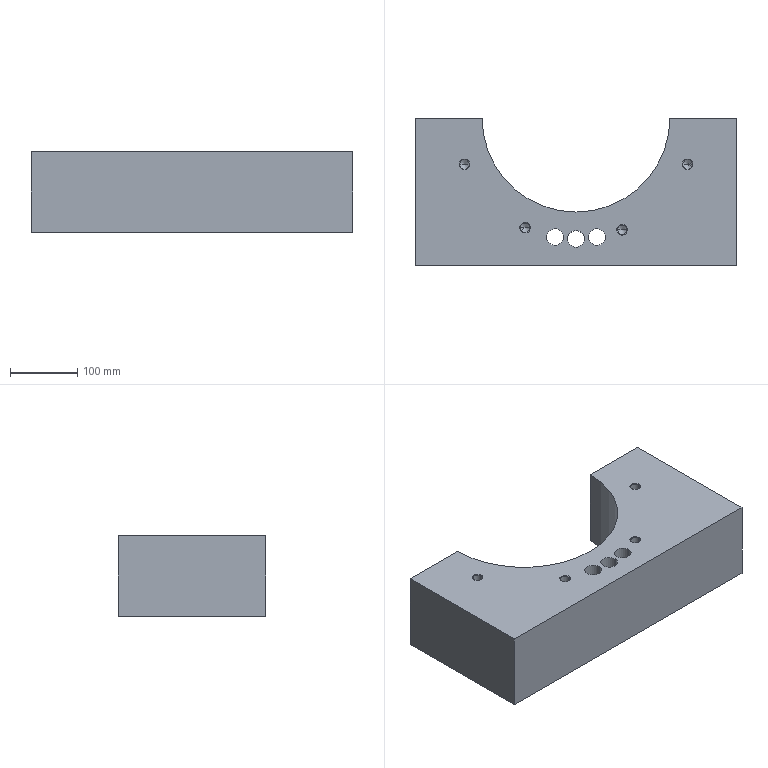Part | SolidWorks | features ICE 2, Extrusion 1, HoleWzd 1, RefAxis 1 | 1 solid | 38 faces | box 480 x 220 x 120 mm | volume 8780124 mm3 | cone 16 | cylinder 15 | plane 7 | commonest cylinder face diameters 14 x8 25 x6 280 x1
STEP:
#1=CARTESIAN_POINT('',(-173.298,41.117,119.14));
#2=VERTEX_POINT('',#1);
#3=CARTESIAN_POINT('',(-159.298,41.117,119.14));
#4=VERTEX_POINT('',#3);
#5=CARTESIAN_POINT('',(-166.298,41.117,119.14));
#6=DIRECTION('',(0.,0.,1.));
#7=DIRECTION('',(1.,0.,0.));
#8=AXIS2_PLACEMENT_3D('',#5,#6,#7);
#9=CIRCLE('',#8,7.);
#10=EDGE_CURVE('',#2,#4,#9,.T.);
#11=ORIENTED_EDGE('',*,*,#10,.F.);
#12=CARTESIAN_POINT('',(-174.323,41.117,120.));
#13=VERTEX_POINT('',#12);
#14=CARTESIAN_POINT('',(-174.323,41.117,120.));
#15=DIRECTION('',(-0.766,0.,0.6428));
#16=VECTOR('',#15,1000.);
#17=LINE('',#14,#16);
#18=EDGE_CURVE('',#2,#13,#17,.T.);
#19=ORIENTED_EDGE('',*,*,#18,.T.);
#20=CARTESIAN_POINT('',(-158.273,41.117,120.));
#21=VERTEX_POINT('',#20);
#22=CARTESIAN_POINT('',(-166.298,41.117,120.));
#23=DIRECTION('',(0.,0.,1.));
#24=DIRECTION('',(1.,0.,0.));
#25=AXIS2_PLACEMENT_3D('',#22,#23,#24);
#26=CIRCLE('',#25,8.025);
#27=EDGE_CURVE('',#13,#21,#26,.T.);
#28=ORIENTED_EDGE('',*,*,#27,.T.);
#29=CARTESIAN_POINT('',(-158.273,41.117,120.));
#30=DIRECTION('',(0.766,0.,0.6428));
#31=VECTOR('',#30,1000.);
#32=LINE('',#29,#31);
#33=EDGE_CURVE('',#4,#21,#32,.T.);
#34=ORIENTED_EDGE('',*,*,#33,.F.);
#35=EDGE_LOOP('',(#11,#19,#28,#34));
#36=FACE_OUTER_BOUND('',#35,.T.);
#37=CARTESIAN_POINT('',(-166.298,41.117,120.));
#38=DIRECTION('',(0.,0.,1.));
#39=DIRECTION('',(1.,0.,0.));
#40=AXIS2_PLACEMENT_3D('',#37,#38,#39);
#41=CONICAL_SURFACE('',#40,8.025,0.8727);
#42=ADVANCED_FACE('',(#36),#41,.F.);
#43=CARTESIAN_POINT('',(-173.298,41.117,88.));
#44=VERTEX_POINT('',#43);
#45=CARTESIAN_POINT('',(-159.298,41.117,88.));
#46=VERTEX_POINT('',#45);
#47=CARTESIAN_POINT('',(-166.298,41.117,88.));
#48=DIRECTION('',(0.,0.,1.));
#49=DIRECTION('',(1.,0.,0.));
#50=AXIS2_PLACEMENT_3D('',#47,#48,#49);
#51=CIRCLE('',#50,7.);
#52=EDGE_CURVE('',#44,#46,#51,.T.);
#53=ORIENTED_EDGE('',*,*,#52,.F.);
#54=CARTESIAN_POINT('',(-173.298,41.117,120.));
#55=DIRECTION('',(0.,0.,1.));
#56=VECTOR('',#55,1000.);
#57=LINE('',#54,#56);
#58=EDGE_CURVE('',#44,#2,#57,.T.);
#59=ORIENTED_EDGE('',*,*,#58,.T.);
#60=ORIENTED_EDGE('',*,*,#10,.T.);
#61=CARTESIAN_POINT('',(-159.298,41.117,120.));
#62=DIRECTION('',(0.,0.,1.));
#63=VECTOR('',#62,1000.);
#64=LINE('',#61,#63);
#65=EDGE_CURVE('',#46,#4,#64,.T.);
#66=ORIENTED_EDGE('',*,*,#65,.F.);
#67=EDGE_LOOP('',(#53,#59,#60,#66));
#68=FACE_OUTER_BOUND('',#67,.T.);
#69=CARTESIAN_POINT('',(-166.298,41.117,120.));
#70=DIRECTION('',(0.,0.,1.));
#71=DIRECTION('',(1.,0.,0.));
#72=AXIS2_PLACEMENT_3D('',#69,#70,#71);
#73=CYLINDRICAL_SURFACE('',#72,7.);
#74=ADVANCED_FACE('',(#68),#73,.F.);
#75=CARTESIAN_POINT('',(-166.298,41.117,83.794));
#76=VERTEX_POINT('',#75);
#77=CARTESIAN_POINT('',(-159.298,41.117,88.));
#78=DIRECTION('',(0.8572,0.,0.515));
#79=VECTOR('',#78,1000.);
#80=LINE('',#77,#79);
#81=EDGE_CURVE('',#76,#46,#80,.T.);
#82=ORIENTED_EDGE('',*,*,#81,.F.);
#83=CARTESIAN_POINT('',(-173.298,41.117,88.));
#84=DIRECTION('',(-0.8572,0.,0.515));
#85=VECTOR('',#84,1000.);
#86=LINE('',#83,#85);
#87=EDGE_CURVE('',#76,#44,#86,.T.);
#88=ORIENTED_EDGE('',*,*,#87,.T.);
#89=ORIENTED_EDGE('',*,*,#52,.T.);
#90=EDGE_LOOP('',(#82,#88,#89));
#91=FACE_OUTER_BOUND('',#90,.T.);
#92=CARTESIAN_POINT('',(-166.298,41.117,88.));
#93=DIRECTION('',(0.,0.,1.));
#94=DIRECTION('',(1.,0.,0.));
#95=AXIS2_PLACEMENT_3D('',#92,#93,#94);
#96=CONICAL_SURFACE('',#95,7.,1.03);
#97=ADVANCED_FACE('',(#91),#96,.F.);
#98=CARTESIAN_POINT('',(159.298,41.117,119.14));
#99=VERTEX_POINT('',#98);
#100=CARTESIAN_POINT('',(173.298,41.117,119.14));
#101=VERTEX_POINT('',#100);
#102=CARTESIAN_POINT('',(166.298,41.117,119.14));
#103=DIRECTION('',(0.,0.,1.));
#104=DIRECTION('',(1.,0.,0.));
#105=AXIS2_PLACEMENT_3D('',#102,#103,#104);
#106=CIRCLE('',#105,7.);
#107=EDGE_CURVE('',#99,#101,#106,.T.);
#108=ORIENTED_EDGE('',*,*,#107,.F.);
#109=CARTESIAN_POINT('',(158.273,41.117,120.));
#110=VERTEX_POINT('',#109);
#111=CARTESIAN_POINT('',(158.273,41.117,120.));
#112=DIRECTION('',(-0.766,0.,0.6428));
#113=VECTOR('',#112,1000.);
#114=LINE('',#111,#113);
#115=EDGE_CURVE('',#99,#110,#114,.T.);
#116=ORIENTED_EDGE('',*,*,#115,.T.);
#117=CARTESIAN_POINT('',(174.323,41.117,120.));
#118=VERTEX_POINT('',#117);
#119=CARTESIAN_POINT('',(166.298,41.117,120.));
#120=DIRECTION('',(0.,0.,1.));
#121=DIRECTION('',(1.,0.,0.));
#122=AXIS2_PLACEMENT_3D('',#119,#120,#121);
#123=CIRCLE('',#122,8.025);
#124=EDGE_CURVE('',#110,#118,#123,.T.);
#125=ORIENTED_EDGE('',*,*,#124,.T.);
#126=CARTESIAN_POINT('',(174.323,41.117,120.));
#127=DIRECTION('',(0.766,0.,0.6428));
#128=VECTOR('',#127,1000.);
#129=LINE('',#126,#128);
#130=EDGE_CURVE('',#101,#118,#129,.T.);
#131=ORIENTED_EDGE('',*,*,#130,.F.);
#132=EDGE_LOOP('',(#108,#116,#125,#131));
#133=FACE_OUTER_BOUND('',#132,.T.);
#134=CARTESIAN_POINT('',(166.298,41.117,120.));
#135=DIRECTION('',(0.,0.,1.));
#136=DIRECTION('',(1.,0.,0.));
#137=AXIS2_PLACEMENT_3D('',#134,#135,#136);
#138=CONICAL_SURFACE('',#137,8.025,0.8727);
#139=ADVANCED_FACE('',(#133),#138,.F.);
#140=CARTESIAN_POINT('',(159.298,41.117,88.));
#141=VERTEX_POINT('',#140);
#142=CARTESIAN_POINT('',(173.298,41.117,88.));
#143=VERTEX_POINT('',#142);
#144=CARTESIAN_POINT('',(166.298,41.117,88.));
#145=DIRECTION('',(0.,0.,1.));
#146=DIRECTION('',(1.,0.,0.));
#147=AXIS2_PLACEMENT_3D('',#144,#145,#146);
#148=CIRCLE('',#147,7.);
#149=EDGE_CURVE('',#141,#143,#148,.T.);
#150=ORIENTED_EDGE('',*,*,#149,.F.);
#151=CARTESIAN_POINT('',(159.298,41.117,120.));
#152=DIRECTION('',(0.,0.,1.));
#153=VECTOR('',#152,1000.);
#154=LINE('',#151,#153);
#155=EDGE_CURVE('',#141,#99,#154,.T.);
#156=ORIENTED_EDGE('',*,*,#155,.T.);
#157=ORIENTED_EDGE('',*,*,#107,.T.);
#158=CARTESIAN_POINT('',(173.298,41.117,120.));
#159=DIRECTION('',(0.,0.,1.));
#160=VECTOR('',#159,1000.);
#161=LINE('',#158,#160);
#162=EDGE_CURVE('',#143,#101,#161,.T.);
#163=ORIENTED_EDGE('',*,*,#162,.F.);
#164=EDGE_LOOP('',(#150,#156,#157,#163));
#165=FACE_OUTER_BOUND('',#164,.T.);
#166=CARTESIAN_POINT('',(166.298,41.117,120.));
#167=DIRECTION('',(0.,0.,1.));
#168=DIRECTION('',(1.,0.,0.));
#169=AXIS2_PLACEMENT_3D('',#166,#167,#168);
#170=CYLINDRICAL_SURFACE('',#169,7.);
#171=ADVANCED_FACE('',(#165),#170,.F.);
#172=CARTESIAN_POINT('',(166.298,41.117,83.794));
#173=VERTEX_POINT('',#172);
#174=CARTESIAN_POINT('',(173.298,41.117,88.));
#175=DIRECTION('',(0.8572,0.,0.515));
#176=VECTOR('',#175,1000.);
#177=LINE('',#174,#176);
#178=EDGE_CURVE('',#173,#143,#177,.T.);
#179=ORIENTED_EDGE('',*,*,#178,.F.);
#180=CARTESIAN_POINT('',(159.298,41.117,88.));
#181=DIRECTION('',(-0.8572,0.,0.515));
#182=VECTOR('',#181,1000.);
#183=LINE('',#180,#182);
#184=EDGE_CURVE('',#173,#141,#183,.T.);
#185=ORIENTED_EDGE('',*,*,#184,.T.);
#186=ORIENTED_EDGE('',*,*,#149,.T.);
#187=EDGE_LOOP('',(#179,#185,#186));
#188=FACE_OUTER_BOUND('',#187,.T.);
#189=CARTESIAN_POINT('',(166.298,41.117,88.));
#190=DIRECTION('',(0.,0.,1.));
#191=DIRECTION('',(1.,0.,0.));
#192=AXIS2_PLACEMENT_3D('',#189,#190,#191);
#193=CONICAL_SURFACE('',#192,7.,1.03);
#194=ADVANCED_FACE('',(#188),#193,.F.);
#195=CARTESIAN_POINT('',(61.883,-56.298,119.14));
#196=VERTEX_POINT('',#195);
#197=CARTESIAN_POINT('',(75.883,-56.298,119.14));
#198=VERTEX_POINT('',#197);
#199=CARTESIAN_POINT('',(68.883,-56.298,119.14));
#200=DIRECTION('',(0.,0.,1.));
#201=DIRECTION('',(1.,0.,0.));
#202=AXIS2_PLACEMENT_3D('',#199,#200,#201);
#203=CIRCLE('',#202,7.);
#204=EDGE_CURVE('',#196,#198,#203,.T.);
#205=ORIENTED_EDGE('',*,*,#204,.F.);
#206=CARTESIAN_POINT('',(60.858,-56.298,120.));
#207=VERTEX_POINT('',#206);
#208=CARTESIAN_POINT('',(60.858,-56.298,120.));
#209=DIRECTION('',(-0.766,0.,0.6428));
#210=VECTOR('',#209,1000.);
#211=LINE('',#208,#210);
#212=EDGE_CURVE('',#196,#207,#211,.T.);
#213=ORIENTED_EDGE('',*,*,#212,.T.);
#214=CARTESIAN_POINT('',(76.908,-56.298,120.));
#215=VERTEX_POINT('',#214);
#216=CARTESIAN_POINT('',(68.883,-56.298,120.));
#217=DIRECTION('',(0.,0.,1.));
#218=DIRECTION('',(1.,0.,0.));
#219=AXIS2_PLACEMENT_3D('',#216,#217,#218);
#220=CIRCLE('',#219,8.025);
#221=EDGE_CURVE('',#207,#215,#220,.T.);
#222=ORIENTED_EDGE('',*,*,#221,.T.);
#223=CARTESIAN_POINT('',(76.908,-56.298,120.));
#224=DIRECTION('',(0.766,0.,0.6428));
#225=VECTOR('',#224,1000.);
#226=LINE('',#223,#225);
#227=EDGE_CURVE('',#198,#215,#226,.T.);
#228=ORIENTED_EDGE('',*,*,#227,.F.);
#229=EDGE_LOOP('',(#205,#213,#222,#228));
#230=FACE_OUTER_BOUND('',#229,.T.);
#231=CARTESIAN_POINT('',(68.883,-56.298,120.));
#232=DIRECTION('',(0.,0.,1.));
#233=DIRECTION('',(1.,0.,0.));
#234=AXIS2_PLACEMENT_3D('',#231,#232,#233);
#235=CONICAL_SURFACE('',#234,8.025,0.8727);
#236=ADVANCED_FACE('',(#230),#235,.F.);
#237=CARTESIAN_POINT('',(61.883,-56.298,88.));
#238=VERTEX_POINT('',#237);
#239=CARTESIAN_POINT('',(75.883,-56.298,88.));
#240=VERTEX_POINT('',#239);
#241=CARTESIAN_POINT('',(68.883,-56.298,88.));
#242=DIRECTION('',(0.,0.,1.));
#243=DIRECTION('',(1.,0.,0.));
#244=AXIS2_PLACEMENT_3D('',#241,#242,#243);
#245=CIRCLE('',#244,7.);
#246=EDGE_CURVE('',#238,#240,#245,.T.);
#247=ORIENTED_EDGE('',*,*,#246,.F.);
#248=CARTESIAN_POINT('',(61.883,-56.298,120.));
#249=DIRECTION('',(0.,0.,1.));
#250=VECTOR('',#249,1000.);
#251=LINE('',#248,#250);
#252=EDGE_CURVE('',#238,#196,#251,.T.);
#253=ORIENTED_EDGE('',*,*,#252,.T.);
#254=ORIENTED_EDGE('',*,*,#204,.T.);
#255=CARTESIAN_POINT('',(75.883,-56.298,120.));
#256=DIRECTION('',(0.,0.,1.));
#257=VECTOR('',#256,1000.);
#258=LINE('',#255,#257);
#259=EDGE_CURVE('',#240,#198,#258,.T.);
#260=ORIENTED_EDGE('',*,*,#259,.F.);
#261=EDGE_LOOP('',(#247,#253,#254,#260));
#262=FACE_OUTER_BOUND('',#261,.T.);
#263=CARTESIAN_POINT('',(68.883,-56.298,120.));
#264=DIRECTION('',(0.,0.,1.));
#265=DIRECTION('',(1.,0.,0.));
#266=AXIS2_PLACEMENT_3D('',#263,#264,#265);
#267=CYLINDRICAL_SURFACE('',#266,7.);
#268=ADVANCED_FACE('',(#262),#267,.F.);
#269=CARTESIAN_POINT('',(68.883,-56.298,83.794));
#270=VERTEX_POINT('',#269);
#271=CARTESIAN_POINT('',(75.883,-56.298,88.));
#272=DIRECTION('',(0.8572,0.,0.515));
#273=VECTOR('',#272,1000.);
#274=LINE('',#271,#273);
#275=EDGE_CURVE('',#270,#240,#274,.T.);
#276=ORIENTED_EDGE('',*,*,#275,.F.);
#277=CARTESIAN_POINT('',(61.883,-56.298,88.));
#278=DIRECTION('',(-0.8572,0.,0.515));
#279=VECTOR('',#278,1000.);
#280=LINE('',#277,#279);
#281=EDGE_CURVE('',#270,#238,#280,.T.);
#282=ORIENTED_EDGE('',*,*,#281,.T.);
#283=ORIENTED_EDGE('',*,*,#246,.T.);
#284=EDGE_LOOP('',(#276,#282,#283));
#285=FACE_OUTER_BOUND('',#284,.T.);
#286=CARTESIAN_POINT('',(68.883,-56.298,88.));
#287=DIRECTION('',(0.,0.,1.));
#288=DIRECTION('',(1.,0.,0.));
#289=AXIS2_PLACEMENT_3D('',#286,#287,#288);
#290=CONICAL_SURFACE('',#289,7.,1.03);
#291=ADVANCED_FACE('',(#285),#290,.F.);
#292=CARTESIAN_POINT('',(-82.868,-53.23,119.14));
#293=VERTEX_POINT('',#292);
#294=CARTESIAN_POINT('',(-68.868,-53.23,119.14));
#295=VERTEX_POINT('',#294);
#296=CARTESIAN_POINT('',(-75.868,-53.23,119.14));
#297=DIRECTION('',(0.,0.,1.));
#298=DIRECTION('',(1.,0.,0.));
#299=AXIS2_PLACEMENT_3D('',#296,#297,#298);
#300=CIRCLE('',#299,7.);
#301=EDGE_CURVE('',#293,#295,#300,.T.);
#302=ORIENTED_EDGE('',*,*,#301,.F.);
#303=CARTESIAN_POINT('',(-83.893,-53.23,120.));
#304=VERTEX_POINT('',#303);
#305=CARTESIAN_POINT('',(-83.893,-53.23,120.));
#306=DIRECTION('',(-0.766,0.,0.6428));
#307=VECTOR('',#306,1000.);
#308=LINE('',#305,#307);
#309=EDGE_CURVE('',#293,#304,#308,.T.);
#310=ORIENTED_EDGE('',*,*,#309,.T.);
#311=CARTESIAN_POINT('',(-67.843,-53.23,120.));
#312=VERTEX_POINT('',#311);
#313=CARTESIAN_POINT('',(-75.868,-53.23,120.));
#314=DIRECTION('',(0.,0.,1.));
#315=DIRECTION('',(1.,0.,0.));
#316=AXIS2_PLACEMENT_3D('',#313,#314,#315);
#317=CIRCLE('',#316,8.025);
#318=EDGE_CURVE('',#304,#312,#317,.T.);
#319=ORIENTED_EDGE('',*,*,#318,.T.);
#320=CARTESIAN_POINT('',(-67.843,-53.23,120.));
#321=DIRECTION('',(0.766,0.,0.6428));
#322=VECTOR('',#321,1000.);
#323=LINE('',#320,#322);
#324=EDGE_CURVE('',#295,#312,#323,.T.);
#325=ORIENTED_EDGE('',*,*,#324,.F.);
#326=EDGE_LOOP('',(#302,#310,#319,#325));
#327=FACE_OUTER_BOUND('',#326,.T.);
#328=CARTESIAN_POINT('',(-75.868,-53.23,120.));
#329=DIRECTION('',(0.,0.,1.));
#330=DIRECTION('',(1.,0.,0.));
#331=AXIS2_PLACEMENT_3D('',#328,#329,#330);
#332=CONICAL_SURFACE('',#331,8.025,0.8727);
#333=ADVANCED_FACE('',(#327),#332,.F.);
#334=CARTESIAN_POINT('',(-82.868,-53.23,88.));
#335=VERTEX_POINT('',#334);
#336=CARTESIAN_POINT('',(-68.868,-53.23,88.));
#337=VERTEX_POINT('',#336);
#338=CARTESIAN_POINT('',(-75.868,-53.23,88.));
#339=DIRECTION('',(0.,0.,1.));
#340=DIRECTION('',(1.,0.,0.));
#341=AXIS2_PLACEMENT_3D('',#338,#339,#340);
#342=CIRCLE('',#341,7.);
#343=EDGE_CURVE('',#335,#337,#342,.T.);
#344=ORIENTED_EDGE('',*,*,#343,.F.);
#345=CARTESIAN_POINT('',(-82.868,-53.23,120.));
#346=DIRECTION('',(0.,0.,1.));
#347=VECTOR('',#346,1000.);
#348=LINE('',#345,#347);
#349=EDGE_CURVE('',#335,#293,#348,.T.);
#350=ORIENTED_EDGE('',*,*,#349,.T.);
#351=ORIENTED_EDGE('',*,*,#301,.T.);
#352=CARTESIAN_POINT('',(-68.868,-53.23,120.));
#353=DIRECTION('',(0.,0.,1.));
#354=VECTOR('',#353,1000.);
#355=LINE('',#352,#354);
#356=EDGE_CURVE('',#337,#295,#355,.T.);
#357=ORIENTED_EDGE('',*,*,#356,.F.);
#358=EDGE_LOOP('',(#344,#350,#351,#357));
#359=FACE_OUTER_BOUND('',#358,.T.);
#360=CARTESIAN_POINT('',(-75.868,-53.23,120.));
#361=DIRECTION('',(0.,0.,1.));
#362=DIRECTION('',(1.,0.,0.));
#363=AXIS2_PLACEMENT_3D('',#360,#361,#362);
#364=CYLINDRICAL_SURFACE('',#363,7.);
#365=ADVANCED_FACE('',(#359),#364,.F.);
#366=CARTESIAN_POINT('',(-75.868,-53.23,83.794));
#367=VERTEX_POINT('',#366);
#368=CARTESIAN_POINT('',(-68.868,-53.23,88.));
#369=DIRECTION('',(0.8572,0.,0.515));
#370=VECTOR('',#369,1000.);
#371=LINE('',#368,#370);
#372=EDGE_CURVE('',#367,#337,#371,.T.);
#373=ORIENTED_EDGE('',*,*,#372,.F.);
#374=CARTESIAN_POINT('',(-82.868,-53.23,88.));
#375=DIRECTION('',(-0.8572,0.,0.515));
#376=VECTOR('',#375,1000.);
#377=LINE('',#374,#376);
#378=EDGE_CURVE('',#367,#335,#377,.T.);
#379=ORIENTED_EDGE('',*,*,#378,.T.);
#380=ORIENTED_EDGE('',*,*,#343,.T.);
#381=EDGE_LOOP('',(#373,#379,#380));
#382=FACE_OUTER_BOUND('',#381,.T.);
#383=CARTESIAN_POINT('',(-75.868,-53.23,88.));
#384=DIRECTION('',(0.,0.,1.));
#385=DIRECTION('',(1.,0.,0.));
#386=AXIS2_PLACEMENT_3D('',#383,#384,#385);
#387=CONICAL_SURFACE('',#386,7.,1.03);
#388=ADVANCED_FACE('',(#382),#387,.F.);
#389=CARTESIAN_POINT('',(18.757,-67.265,0.));
#390=VERTEX_POINT('',#389);
#391=CARTESIAN_POINT('',(43.757,-67.265,0.));
#392=VERTEX_POINT('',#391);
#393=CARTESIAN_POINT('',(31.257,-67.265,0.));
#394=DIRECTION('',(0.,0.,1.));
#395=DIRECTION('',(-1.,0.,0.));
#396=AXIS2_PLACEMENT_3D('',#393,#394,#395);
#397=CIRCLE('',#396,12.5);
#398=EDGE_CURVE('',#390,#392,#397,.T.);
#399=ORIENTED_EDGE('',*,*,#398,.F.);
#400=CARTESIAN_POINT('',(18.757,-67.265,120.));
#401=VERTEX_POINT('',#400);
#402=CARTESIAN_POINT('',(18.757,-67.265,0.));
#403=DIRECTION('',(0.,0.,1.));
#404=VECTOR('',#403,1000.);
#405=LINE('',#402,#404);
#406=EDGE_CURVE('',#390,#401,#405,.T.);
#407=ORIENTED_EDGE('',*,*,#406,.T.);
#408=CARTESIAN_POINT('',(43.757,-67.265,120.));
#409=VERTEX_POINT('',#408);
#410=CARTESIAN_POINT('',(31.257,-67.265,120.));
#411=DIRECTION('',(0.,0.,1.));
#412=DIRECTION('',(1.,0.,0.));
#413=AXIS2_PLACEMENT_3D('',#410,#411,#412);
#414=CIRCLE('',#413,12.5);
#415=EDGE_CURVE('',#401,#409,#414,.T.);
#416=ORIENTED_EDGE('',*,*,#415,.T.);
#417=CARTESIAN_POINT('',(43.757,-67.265,0.));
#418=DIRECTION('',(0.,0.,1.));
#419=VECTOR('',#418,1000.);
#420=LINE('',#417,#419);
#421=EDGE_CURVE('',#392,#409,#420,.T.);
#422=ORIENTED_EDGE('',*,*,#421,.F.);
#423=EDGE_LOOP('',(#399,#407,#416,#422));
#424=FACE_OUTER_BOUND('',#423,.T.);
#425=CARTESIAN_POINT('',(31.257,-67.265,0.));
#426=DIRECTION('',(0.,0.,1.));
#427=DIRECTION('',(1.,0.,0.));
#428=AXIS2_PLACEMENT_3D('',#425,#426,#427);
#429=CYLINDRICAL_SURFACE('',#428,12.5);
#430=ADVANCED_FACE('',(#424),#429,.F.);
#431=CARTESIAN_POINT('',(-43.757,-67.265,0.));
#432=VERTEX_POINT('',#431);
#433=CARTESIAN_POINT('',(-18.757,-67.265,0.));
#434=VERTEX_POINT('',#433);
#435=CARTESIAN_POINT('',(-31.257,-67.265,0.));
#436=DIRECTION('',(0.,0.,1.));
#437=DIRECTION('',(1.,0.,0.));
#438=AXIS2_PLACEMENT_3D('',#435,#436,#437);
#439=CIRCLE('',#438,12.5);
#440=EDGE_CURVE('',#432,#434,#439,.T.);
#441=ORIENTED_EDGE('',*,*,#440,.F.);
#442=CARTESIAN_POINT('',(-43.757,-67.265,120.));
#443=VERTEX_POINT('',#442);
#444=CARTESIAN_POINT('',(-43.757,-67.265,0.));
#445=DIRECTION('',(0.,0.,1.));
#446=VECTOR('',#445,1000.);
#447=LINE('',#444,#446);
#448=EDGE_CURVE('',#432,#443,#447,.T.);
#449=ORIENTED_EDGE('',*,*,#448,.T.);
#450=CARTESIAN_POINT('',(-18.757,-67.265,120.));
#451=VERTEX_POINT('',#450);
#452=CARTESIAN_POINT('',(-31.257,-67.265,120.));
#453=DIRECTION('',(0.,0.,1.));
#454=DIRECTION('',(1.,0.,0.));
#455=AXIS2_PLACEMENT_3D('',#452,#453,#454);
#456=CIRCLE('',#455,12.5);
#457=EDGE_CURVE('',#443,#451,#456,.T.);
#458=ORIENTED_EDGE('',*,*,#457,.T.);
#459=CARTESIAN_POINT('',(-18.757,-67.265,0.));
#460=DIRECTION('',(0.,0.,1.));
#461=VECTOR('',#460,1000.);
#462=LINE('',#459,#461);
#463=EDGE_CURVE('',#434,#451,#462,.T.);
#464=ORIENTED_EDGE('',*,*,#463,.F.);
#465=EDGE_LOOP('',(#441,#449,#458,#464));
#466=FACE_OUTER_BOUND('',#465,.T.);
#467=CARTESIAN_POINT('',(-31.257,-67.265,0.));
#468=DIRECTION('',(0.,0.,1.));
#469=DIRECTION('',(1.,0.,0.));
#470=AXIS2_PLACEMENT_3D('',#467,#468,#469);
#471=CYLINDRICAL_SURFACE('',#470,12.5);
#472=ADVANCED_FACE('',(#466),#471,.F.);
#473=CARTESIAN_POINT('',(-12.5,-70.,0.));
#474=VERTEX_POINT('',#473);
#475=CARTESIAN_POINT('',(12.5,-70.,0.));
#476=VERTEX_POINT('',#475);
#477=CARTESIAN_POINT('',(0.,-70.,0.));
#478=DIRECTION('',(0.,0.,1.));
#479=DIRECTION('',(1.,0.,0.));
#480=AXIS2_PLACEMENT_3D('',#477,#478,#479);
#481=CIRCLE('',#480,12.5);
#482=EDGE_CURVE('',#474,#476,#481,.T.);
#483=ORIENTED_EDGE('',*,*,#482,.F.);
#484=CARTESIAN_POINT('',(-12.5,-70.,120.));
#485=VERTEX_POINT('',#484);
#486=CARTESIAN_POINT('',(-12.5,-70.,0.));
#487=DIRECTION('',(0.,0.,1.));
#488=VECTOR('',#487,1000.);
#489=LINE('',#486,#488);
#490=EDGE_CURVE('',#474,#485,#489,.T.);
#491=ORIENTED_EDGE('',*,*,#490,.T.);
#492=CARTESIAN_POINT('',(12.5,-70.,120.));
#493=VERTEX_POINT('',#492);
#494=CARTESIAN_POINT('',(0.,-70.,120.));
#495=DIRECTION('',(0.,0.,1.));
#496=DIRECTION('',(1.,0.,0.));
#497=AXIS2_PLACEMENT_3D('',#494,#495,#496);
#498=CIRCLE('',#497,12.5);
#499=EDGE_CURVE('',#485,#493,#498,.T.);
#500=ORIENTED_EDGE('',*,*,#499,.T.);
#501=CARTESIAN_POINT('',(12.5,-70.,0.));
#502=DIRECTION('',(0.,0.,1.));
#503=VECTOR('',#502,1000.);
#504=LINE('',#501,#503);
#505=EDGE_CURVE('',#476,#493,#504,.T.);
#506=ORIENTED_EDGE('',*,*,#505,.F.);
#507=EDGE_LOOP('',(#483,#491,#500,#506));
#508=FACE_OUTER_BOUND('',#507,.T.);
#509=CARTESIAN_POINT('',(0.,-70.,0.));
#510=DIRECTION('',(0.,0.,1.));
#511=DIRECTION('',(1.,0.,0.));
#512=AXIS2_PLACEMENT_3D('',#509,#510,#511);
#513=CYLINDRICAL_SURFACE('',#512,12.5);
#514=ADVANCED_FACE('',(#508),#513,.F.);
#515=CARTESIAN_POINT('',(240.,110.,0.));
#516=VERTEX_POINT('',#515);
#517=CARTESIAN_POINT('',(140.,110.,0.));
#518=VERTEX_POINT('',#517);
#519=CARTESIAN_POINT('',(-240.,110.,0.));
#520=DIRECTION('',(-1.,0.,0.));
#521=VECTOR('',#520,1000.);
#522=LINE('',#519,#521);
#523=EDGE_CURVE('',#516,#518,#522,.T.);
#524=ORIENTED_EDGE('',*,*,#523,.T.);
#525=CARTESIAN_POINT('',(140.,110.,120.));
#526=VERTEX_POINT('',#525);
#527=CARTESIAN_POINT('',(140.,110.,0.));
#528=DIRECTION('',(0.,0.,1.));
#529=VECTOR('',#528,1000.);
#530=LINE('',#527,#529);
#531=EDGE_CURVE('',#518,#526,#530,.T.);
#532=ORIENTED_EDGE('',*,*,#531,.T.);
#533=CARTESIAN_POINT('',(240.,110.,120.));
#534=VERTEX_POINT('',#533);
#535=CARTESIAN_POINT('',(-240.,110.,120.));
#536=DIRECTION('',(-1.,0.,0.));
#537=VECTOR('',#536,1000.);
#538=LINE('',#535,#537);
#539=EDGE_CURVE('',#534,#526,#538,.T.);
#540=ORIENTED_EDGE('',*,*,#539,.F.);
#541=CARTESIAN_POINT('',(240.,110.,120.));
#542=DIRECTION('',(0.,0.,-1.));
#543=VECTOR('',#542,1000.);
#544=LINE('',#541,#543);
#545=EDGE_CURVE('',#534,#516,#544,.T.);
#546=ORIENTED_EDGE('',*,*,#545,.T.);
#547=EDGE_LOOP('',(#524,#532,#540,#546));
#548=FACE_OUTER_BOUND('',#547,.T.);
#549=CARTESIAN_POINT('',(-240.,110.,120.));
#550=DIRECTION('',(0.,-1.,0.));
#551=DIRECTION('',(0.,0.,-1.));
#552=AXIS2_PLACEMENT_3D('',#549,#550,#551);
#553=PLANE('',#552);
#554=ADVANCED_FACE('',(#548),#553,.F.);
#555=CARTESIAN_POINT('',(240.,-110.,0.));
#556=VERTEX_POINT('',#555);
#557=CARTESIAN_POINT('',(240.,110.,0.));
#558=DIRECTION('',(0.,1.,0.));
#559=VECTOR('',#558,1000.);
#560=LINE('',#557,#559);
#561=EDGE_CURVE('',#556,#516,#560,.T.);
#562=ORIENTED_EDGE('',*,*,#561,.T.);
#563=ORIENTED_EDGE('',*,*,#545,.F.);
#564=CARTESIAN_POINT('',(240.,-110.,120.));
#565=VERTEX_POINT('',#564);
#566=CARTESIAN_POINT('',(240.,110.,120.));
#567=DIRECTION('',(0.,1.,0.));
#568=VECTOR('',#567,1000.);
#569=LINE('',#566,#568);
#570=EDGE_CURVE('',#565,#534,#569,.T.);
#571=ORIENTED_EDGE('',*,*,#570,.F.);
#572=CARTESIAN_POINT('',(240.,-110.,120.));
#573=DIRECTION('',(0.,0.,-1.));
#574=VECTOR('',#573,1000.);
#575=LINE('',#572,#574);
#576=EDGE_CURVE('',#565,#556,#575,.T.);
#577=ORIENTED_EDGE('',*,*,#576,.T.);
#578=EDGE_LOOP('',(#562,#563,#571,#577));
#579=FACE_OUTER_BOUND('',#578,.T.);
#580=CARTESIAN_POINT('',(240.,110.,120.));
#581=DIRECTION('',(-1.,0.,0.));
#582=DIRECTION('',(0.,0.,1.));
#583=AXIS2_PLACEMENT_3D('',#580,#581,#582);
#584=PLANE('',#583);
#585=ADVANCED_FACE('',(#579),#584,.F.);
#586=CARTESIAN_POINT('',(-140.,110.,120.));
#587=VERTEX_POINT('',#586);
#588=CARTESIAN_POINT('',(-240.,110.,120.));
#589=VERTEX_POINT('',#588);
#590=CARTESIAN_POINT('',(-240.,110.,120.));
#591=DIRECTION('',(-1.,0.,0.));
#592=VECTOR('',#591,1000.);
#593=LINE('',#590,#592);
#594=EDGE_CURVE('',#587,#589,#593,.T.);
#595=ORIENTED_EDGE('',*,*,#594,.F.);
#596=CARTESIAN_POINT('',(-140.,110.,0.));
#597=VERTEX_POINT('',#596);
#598=CARTESIAN_POINT('',(-140.,110.,0.));
#599=DIRECTION('',(0.,0.,-1.));
#600=VECTOR('',#599,1000.);
#601=LINE('',#598,#600);
#602=EDGE_CURVE('',#587,#597,#601,.T.);
#603=ORIENTED_EDGE('',*,*,#602,.T.);
#604=CARTESIAN_POINT('',(-240.,110.,0.));
#605=VERTEX_POINT('',#604);
#606=CARTESIAN_POINT('',(-240.,110.,0.));
#607=DIRECTION('',(-1.,0.,0.));
#608=VECTOR('',#607,1000.);
#609=LINE('',#606,#608);
#610=EDGE_CURVE('',#597,#605,#609,.T.);
#611=ORIENTED_EDGE('',*,*,#610,.T.);
#612=CARTESIAN_POINT('',(-240.,110.,120.));
#613=DIRECTION('',(0.,0.,-1.));
#614=VECTOR('',#613,1000.);
#615=LINE('',#612,#614);
#616=EDGE_CURVE('',#589,#605,#615,.T.);
#617=ORIENTED_EDGE('',*,*,#616,.F.);
#618=EDGE_LOOP('',(#595,#603,#611,#617));
#619=FACE_OUTER_BOUND('',#618,.T.);
#620=CARTESIAN_POINT('',(-240.,110.,120.));
#621=DIRECTION('',(0.,-1.,0.));
#622=DIRECTION('',(0.,0.,-1.));
#623=AXIS2_PLACEMENT_3D('',#620,#621,#622);
#624=PLANE('',#623);
#625=ADVANCED_FACE('',(#619),#624,.F.);
#626=CARTESIAN_POINT('',(-240.,-110.,0.));
#627=VERTEX_POINT('',#626);
#628=CARTESIAN_POINT('',(-240.,110.,0.));
#629=DIRECTION('',(0.,-1.,0.));
#630=VECTOR('',#629,1000.);
#631=LINE('',#628,#630);
#632=EDGE_CURVE('',#605,#627,#631,.T.);
#633=ORIENTED_EDGE('',*,*,#632,.T.);
#634=CARTESIAN_POINT('',(-240.,-110.,120.));
#635=VERTEX_POINT('',#634);
#636=CARTESIAN_POINT('',(-240.,-110.,120.));
#637=DIRECTION('',(0.,0.,-1.));
#638=VECTOR('',#637,1000.);
#639=LINE('',#636,#638);
#640=EDGE_CURVE('',#635,#627,#639,.T.);
#641=ORIENTED_EDGE('',*,*,#640,.F.);
#642=CARTESIAN_POINT('',(-240.,110.,120.));
#643=DIRECTION('',(0.,-1.,0.));
#644=VECTOR('',#643,1000.);
#645=LINE('',#642,#644);
#646=EDGE_CURVE('',#589,#635,#645,.T.);
#647=ORIENTED_EDGE('',*,*,#646,.F.);
#648=ORIENTED_EDGE('',*,*,#616,.T.);
#649=EDGE_LOOP('',(#633,#641,#647,#648));
#650=FACE_OUTER_BOUND('',#649,.T.);
#651=CARTESIAN_POINT('',(-240.,110.,120.));
#652=DIRECTION('',(1.,0.,0.));
#653=DIRECTION('',(0.,0.,-1.));
#654=AXIS2_PLACEMENT_3D('',#651,#652,#653);
#655=PLANE('',#654);
#656=ADVANCED_FACE('',(#650),#655,.F.);
#657=CARTESIAN_POINT('',(-240.,-110.,0.));
#658=DIRECTION('',(1.,0.,0.));
#659=VECTOR('',#658,1000.);
#660=LINE('',#657,#659);
#661=EDGE_CURVE('',#627,#556,#660,.T.);
#662=ORIENTED_EDGE('',*,*,#661,.T.);
#663=ORIENTED_EDGE('',*,*,#576,.F.);
#664=CARTESIAN_POINT('',(-240.,-110.,120.));
#665=DIRECTION('',(1.,0.,0.));
#666=VECTOR('',#665,1000.);
#667=LINE('',#664,#666);
#668=EDGE_CURVE('',#635,#565,#667,.T.);
#669=ORIENTED_EDGE('',*,*,#668,.F.);
#670=ORIENTED_EDGE('',*,*,#640,.T.);
#671=EDGE_LOOP('',(#662,#663,#669,#670));
#672=FACE_OUTER_BOUND('',#671,.T.);
#673=CARTESIAN_POINT('',(-240.,-110.,120.));
#674=DIRECTION('',(0.,1.,0.));
#675=DIRECTION('',(0.,0.,1.));
#676=AXIS2_PLACEMENT_3D('',#673,#674,#675);
#677=PLANE('',#676);
#678=ADVANCED_FACE('',(#672),#677,.F.);
#679=CARTESIAN_POINT('',(-166.298,41.117,120.));
#680=DIRECTION('',(0.,0.,1.));
#681=DIRECTION('',(1.,0.,0.));
#682=AXIS2_PLACEMENT_3D('',#679,#680,#681);
#683=CIRCLE('',#682,8.025);
#684=EDGE_CURVE('',#21,#13,#683,.T.);
#685=ORIENTED_EDGE('',*,*,#684,.F.);
#686=ORIENTED_EDGE('',*,*,#27,.F.);
#687=EDGE_LOOP('',(#685,#686));
#688=FACE_BOUND('',#687,.T.);
#689=CARTESIAN_POINT('',(166.298,41.117,120.));
#690=DIRECTION('',(0.,0.,1.));
#691=DIRECTION('',(1.,0.,0.));
#692=AXIS2_PLACEMENT_3D('',#689,#690,#691);
#693=CIRCLE('',#692,8.025);
#694=EDGE_CURVE('',#118,#110,#693,.T.);
#695=ORIENTED_EDGE('',*,*,#694,.F.);
#696=ORIENTED_EDGE('',*,*,#124,.F.);
#697=EDGE_LOOP('',(#695,#696));
#698=FACE_BOUND('',#697,.T.);
#699=CARTESIAN_POINT('',(68.883,-56.298,120.));
#700=DIRECTION('',(0.,0.,1.));
#701=DIRECTION('',(1.,0.,0.));
#702=AXIS2_PLACEMENT_3D('',#699,#700,#701);
#703=CIRCLE('',#702,8.025);
#704=EDGE_CURVE('',#215,#207,#703,.T.);
#705=ORIENTED_EDGE('',*,*,#704,.F.);
#706=ORIENTED_EDGE('',*,*,#221,.F.);
#707=EDGE_LOOP('',(#705,#706));
#708=FACE_BOUND('',#707,.T.);
#709=CARTESIAN_POINT('',(-75.868,-53.23,120.));
#710=DIRECTION('',(0.,0.,1.));
#711=DIRECTION('',(1.,0.,0.));
#712=AXIS2_PLACEMENT_3D('',#709,#710,#711);
#713=CIRCLE('',#712,8.025);
#714=EDGE_CURVE('',#312,#304,#713,.T.);
#715=ORIENTED_EDGE('',*,*,#714,.F.);
#716=ORIENTED_EDGE('',*,*,#318,.F.);
#717=EDGE_LOOP('',(#715,#716));
#718=FACE_BOUND('',#717,.T.);
#719=CARTESIAN_POINT('',(31.257,-67.265,120.));
#720=DIRECTION('',(0.,0.,1.));
#721=DIRECTION('',(1.,0.,0.));
#722=AXIS2_PLACEMENT_3D('',#719,#720,#721);
#723=CIRCLE('',#722,12.5);
#724=EDGE_CURVE('',#409,#401,#723,.T.);
#725=ORIENTED_EDGE('',*,*,#724,.F.);
#726=ORIENTED_EDGE('',*,*,#415,.F.);
#727=EDGE_LOOP('',(#725,#726));
#728=FACE_BOUND('',#727,.T.);
#729=CARTESIAN_POINT('',(-31.257,-67.265,120.));
#730=DIRECTION('',(0.,0.,1.));
#731=DIRECTION('',(1.,0.,0.));
#732=AXIS2_PLACEMENT_3D('',#729,#730,#731);
#733=CIRCLE('',#732,12.5);
#734=EDGE_CURVE('',#451,#443,#733,.T.);
#735=ORIENTED_EDGE('',*,*,#734,.F.);
#736=ORIENTED_EDGE('',*,*,#457,.F.);
#737=EDGE_LOOP('',(#735,#736));
#738=FACE_BOUND('',#737,.T.);
#739=CARTESIAN_POINT('',(0.,-70.,120.));
#740=DIRECTION('',(0.,0.,1.));
#741=DIRECTION('',(1.,0.,0.));
#742=AXIS2_PLACEMENT_3D('',#739,#740,#741);
#743=CIRCLE('',#742,12.5);
#744=EDGE_CURVE('',#493,#485,#743,.T.);
#745=ORIENTED_EDGE('',*,*,#744,.F.);
#746=ORIENTED_EDGE('',*,*,#499,.F.);
#747=EDGE_LOOP('',(#745,#746));
#748=FACE_BOUND('',#747,.T.);
#749=CARTESIAN_POINT('',(0.,110.,120.));
#750=DIRECTION('',(0.,0.,1.));
#751=DIRECTION('',(1.,0.,0.));
#752=AXIS2_PLACEMENT_3D('',#749,#750,#751);
#753=CIRCLE('',#752,140.);
#754=EDGE_CURVE('',#587,#526,#753,.T.);
#755=ORIENTED_EDGE('',*,*,#754,.F.);
#756=ORIENTED_EDGE('',*,*,#594,.T.);
#757=ORIENTED_EDGE('',*,*,#646,.T.);
#758=ORIENTED_EDGE('',*,*,#668,.T.);
#759=ORIENTED_EDGE('',*,*,#570,.T.);
#760=ORIENTED_EDGE('',*,*,#539,.T.);
#761=EDGE_LOOP('',(#755,#756,#757,#758,#759,#760));
#762=FACE_OUTER_BOUND('',#761,.T.);
#763=CARTESIAN_POINT('',(0.,0.,120.));
#764=DIRECTION('',(0.,0.,1.));
#765=DIRECTION('',(1.,0.,0.));
#766=AXIS2_PLACEMENT_3D('',#763,#764,#765);
#767=PLANE('',#766);
#768=ADVANCED_FACE('',(#688,#698,#708,#718,#728,#738,#748,#762),#767,.T.);
#769=CARTESIAN_POINT('',(31.257,-67.265,0.));
#770=DIRECTION('',(0.,0.,1.));
#771=DIRECTION('',(-1.,0.,0.));
#772=AXIS2_PLACEMENT_3D('',#769,#770,#771);
#773=CIRCLE('',#772,12.5);
#774=EDGE_CURVE('',#392,#390,#773,.T.);
#775=ORIENTED_EDGE('',*,*,#774,.T.);
#776=ORIENTED_EDGE('',*,*,#398,.T.);
#777=EDGE_LOOP('',(#775,#776));
#778=FACE_BOUND('',#777,.T.);
#779=CARTESIAN_POINT('',(-31.257,-67.265,0.));
#780=DIRECTION('',(0.,0.,1.));
#781=DIRECTION('',(1.,0.,0.));
#782=AXIS2_PLACEMENT_3D('',#779,#780,#781);
#783=CIRCLE('',#782,12.5);
#784=EDGE_CURVE('',#434,#432,#783,.T.);
#785=ORIENTED_EDGE('',*,*,#784,.T.);
#786=ORIENTED_EDGE('',*,*,#440,.T.);
#787=EDGE_LOOP('',(#785,#786));
#788=FACE_BOUND('',#787,.T.);
#789=CARTESIAN_POINT('',(0.,-70.,0.));
#790=DIRECTION('',(0.,0.,1.));
#791=DIRECTION('',(1.,0.,0.));
#792=AXIS2_PLACEMENT_3D('',#789,#790,#791);
#793=CIRCLE('',#792,12.5);
#794=EDGE_CURVE('',#476,#474,#793,.T.);
#795=ORIENTED_EDGE('',*,*,#794,.T.);
#796=ORIENTED_EDGE('',*,*,#482,.T.);
#797=EDGE_LOOP('',(#795,#796));
#798=FACE_BOUND('',#797,.T.);
#799=ORIENTED_EDGE('',*,*,#610,.F.);
#800=CARTESIAN_POINT('',(0.,110.,0.));
#801=DIRECTION('',(0.,0.,1.));
#802=DIRECTION('',(1.,0.,0.));
#803=AXIS2_PLACEMENT_3D('',#800,#801,#802);
#804=CIRCLE('',#803,140.);
#805=EDGE_CURVE('',#597,#518,#804,.T.);
#806=ORIENTED_EDGE('',*,*,#805,.T.);
#807=ORIENTED_EDGE('',*,*,#523,.F.);
#808=ORIENTED_EDGE('',*,*,#561,.F.);
#809=ORIENTED_EDGE('',*,*,#661,.F.);
#810=ORIENTED_EDGE('',*,*,#632,.F.);
#811=EDGE_LOOP('',(#799,#806,#807,#808,#809,#810));
#812=FACE_OUTER_BOUND('',#811,.T.);
#813=CARTESIAN_POINT('',(0.,0.,0.));
#814=DIRECTION('',(0.,0.,1.));
#815=DIRECTION('',(1.,0.,0.));
#816=AXIS2_PLACEMENT_3D('',#813,#814,#815);
#817=PLANE('',#816);
#818=ADVANCED_FACE('',(#778,#788,#798,#812),#817,.F.);
#819=ORIENTED_EDGE('',*,*,#805,.F.);
#820=ORIENTED_EDGE('',*,*,#602,.F.);
#821=ORIENTED_EDGE('',*,*,#754,.T.);
#822=ORIENTED_EDGE('',*,*,#531,.F.);
#823=EDGE_LOOP('',(#819,#820,#821,#822));
#824=FACE_OUTER_BOUND('',#823,.T.);
#825=CARTESIAN_POINT('',(0.,110.,0.));
#826=DIRECTION('',(0.,0.,1.));
#827=DIRECTION('',(1.,0.,0.));
#828=AXIS2_PLACEMENT_3D('',#825,#826,#827);
#829=CYLINDRICAL_SURFACE('',#828,140.);
#830=ADVANCED_FACE('',(#824),#829,.F.);
#831=ORIENTED_EDGE('',*,*,#490,.F.);
#832=ORIENTED_EDGE('',*,*,#794,.F.);
#833=ORIENTED_EDGE('',*,*,#505,.T.);
#834=ORIENTED_EDGE('',*,*,#744,.T.);
#835=EDGE_LOOP('',(#831,#832,#833,#834));
#836=FACE_OUTER_BOUND('',#835,.T.);
#837=CARTESIAN_POINT('',(0.,-70.,0.));
#838=DIRECTION('',(0.,0.,1.));
#839=DIRECTION('',(1.,0.,0.));
#840=AXIS2_PLACEMENT_3D('',#837,#838,#839);
#841=CYLINDRICAL_SURFACE('',#840,12.5);
#842=ADVANCED_FACE('',(#836),#841,.F.);
#843=ORIENTED_EDGE('',*,*,#448,.F.);
#844=ORIENTED_EDGE('',*,*,#784,.F.);
#845=ORIENTED_EDGE('',*,*,#463,.T.);
#846=ORIENTED_EDGE('',*,*,#734,.T.);
#847=EDGE_LOOP('',(#843,#844,#845,#846));
#848=FACE_OUTER_BOUND('',#847,.T.);
#849=CARTESIAN_POINT('',(-31.257,-67.265,0.));
#850=DIRECTION('',(0.,0.,1.));
#851=DIRECTION('',(1.,0.,0.));
#852=AXIS2_PLACEMENT_3D('',#849,#850,#851);
#853=CYLINDRICAL_SURFACE('',#852,12.5);
#854=ADVANCED_FACE('',(#848),#853,.F.);
#855=ORIENTED_EDGE('',*,*,#406,.F.);
#856=ORIENTED_EDGE('',*,*,#774,.F.);
#857=ORIENTED_EDGE('',*,*,#421,.T.);
#858=ORIENTED_EDGE('',*,*,#724,.T.);
#859=EDGE_LOOP('',(#855,#856,#857,#858));
#860=FACE_OUTER_BOUND('',#859,.T.);
#861=CARTESIAN_POINT('',(31.257,-67.265,0.));
#862=DIRECTION('',(0.,0.,1.));
#863=DIRECTION('',(1.,0.,0.));
#864=AXIS2_PLACEMENT_3D('',#861,#862,#863);
#865=CYLINDRICAL_SURFACE('',#864,12.5);
#866=ADVANCED_FACE('',(#860),#865,.F.);
#867=ORIENTED_EDGE('',*,*,#378,.F.);
#868=ORIENTED_EDGE('',*,*,#372,.T.);
#869=CARTESIAN_POINT('',(-75.868,-53.23,88.));
#870=DIRECTION('',(0.,0.,1.));
#871=DIRECTION('',(1.,0.,0.));
#872=AXIS2_PLACEMENT_3D('',#869,#870,#871);
#873=CIRCLE('',#872,7.);
#874=EDGE_CURVE('',#337,#335,#873,.T.);
#875=ORIENTED_EDGE('',*,*,#874,.T.);
#876=EDGE_LOOP('',(#867,#868,#875));
#877=FACE_OUTER_BOUND('',#876,.T.);
#878=CARTESIAN_POINT('',(-75.868,-53.23,88.));
#879=DIRECTION('',(0.,0.,1.));
#880=DIRECTION('',(1.,0.,0.));
#881=AXIS2_PLACEMENT_3D('',#878,#879,#880);
#882=CONICAL_SURFACE('',#881,7.,1.03);
#883=ADVANCED_FACE('',(#877),#882,.F.);
#884=ORIENTED_EDGE('',*,*,#349,.F.);
#885=ORIENTED_EDGE('',*,*,#874,.F.);
#886=ORIENTED_EDGE('',*,*,#356,.T.);
#887=CARTESIAN_POINT('',(-75.868,-53.23,119.14));
#888=DIRECTION('',(0.,0.,1.));
#889=DIRECTION('',(1.,0.,0.));
#890=AXIS2_PLACEMENT_3D('',#887,#888,#889);
#891=CIRCLE('',#890,7.);
#892=EDGE_CURVE('',#295,#293,#891,.T.);
#893=ORIENTED_EDGE('',*,*,#892,.T.);
#894=EDGE_LOOP('',(#884,#885,#886,#893));
#895=FACE_OUTER_BOUND('',#894,.T.);
#896=CARTESIAN_POINT('',(-75.868,-53.23,120.));
#897=DIRECTION('',(0.,0.,1.));
#898=DIRECTION('',(1.,0.,0.));
#899=AXIS2_PLACEMENT_3D('',#896,#897,#898);
#900=CYLINDRICAL_SURFACE('',#899,7.);
#901=ADVANCED_FACE('',(#895),#900,.F.);
#902=ORIENTED_EDGE('',*,*,#309,.F.);
#903=ORIENTED_EDGE('',*,*,#892,.F.);
#904=ORIENTED_EDGE('',*,*,#324,.T.);
#905=ORIENTED_EDGE('',*,*,#714,.T.);
#906=EDGE_LOOP('',(#902,#903,#904,#905));
#907=FACE_OUTER_BOUND('',#906,.T.);
#908=CARTESIAN_POINT('',(-75.868,-53.23,120.));
#909=DIRECTION('',(0.,0.,1.));
#910=DIRECTION('',(1.,0.,0.));
#911=AXIS2_PLACEMENT_3D('',#908,#909,#910);
#912=CONICAL_SURFACE('',#911,8.025,0.8727);
#913=ADVANCED_FACE('',(#907),#912,.F.);
#914=ORIENTED_EDGE('',*,*,#281,.F.);
#915=ORIENTED_EDGE('',*,*,#275,.T.);
#916=CARTESIAN_POINT('',(68.883,-56.298,88.));
#917=DIRECTION('',(0.,0.,1.));
#918=DIRECTION('',(1.,0.,0.));
#919=AXIS2_PLACEMENT_3D('',#916,#917,#918);
#920=CIRCLE('',#919,7.);
#921=EDGE_CURVE('',#240,#238,#920,.T.);
#922=ORIENTED_EDGE('',*,*,#921,.T.);
#923=EDGE_LOOP('',(#914,#915,#922));
#924=FACE_OUTER_BOUND('',#923,.T.);
#925=CARTESIAN_POINT('',(68.883,-56.298,88.));
#926=DIRECTION('',(0.,0.,1.));
#927=DIRECTION('',(1.,0.,0.));
#928=AXIS2_PLACEMENT_3D('',#925,#926,#927);
#929=CONICAL_SURFACE('',#928,7.,1.03);
#930=ADVANCED_FACE('',(#924),#929,.F.);
#931=ORIENTED_EDGE('',*,*,#252,.F.);
#932=ORIENTED_EDGE('',*,*,#921,.F.);
#933=ORIENTED_EDGE('',*,*,#259,.T.);
#934=CARTESIAN_POINT('',(68.883,-56.298,119.14));
#935=DIRECTION('',(0.,0.,1.));
#936=DIRECTION('',(1.,0.,0.));
#937=AXIS2_PLACEMENT_3D('',#934,#935,#936);
#938=CIRCLE('',#937,7.);
#939=EDGE_CURVE('',#198,#196,#938,.T.);
#940=ORIENTED_EDGE('',*,*,#939,.T.);
#941=EDGE_LOOP('',(#931,#932,#933,#940));
#942=FACE_OUTER_BOUND('',#941,.T.);
#943=CARTESIAN_POINT('',(68.883,-56.298,120.));
#944=DIRECTION('',(0.,0.,1.));
#945=DIRECTION('',(1.,0.,0.));
#946=AXIS2_PLACEMENT_3D('',#943,#944,#945);
#947=CYLINDRICAL_SURFACE('',#946,7.);
#948=ADVANCED_FACE('',(#942),#947,.F.);
#949=ORIENTED_EDGE('',*,*,#212,.F.);
#950=ORIENTED_EDGE('',*,*,#939,.F.);
#951=ORIENTED_EDGE('',*,*,#227,.T.);
#952=ORIENTED_EDGE('',*,*,#704,.T.);
#953=EDGE_LOOP('',(#949,#950,#951,#952));
#954=FACE_OUTER_BOUND('',#953,.T.);
#955=CARTESIAN_POINT('',(68.883,-56.298,120.));
#956=DIRECTION('',(0.,0.,1.));
#957=DIRECTION('',(1.,0.,0.));
#958=AXIS2_PLACEMENT_3D('',#955,#956,#957);
#959=CONICAL_SURFACE('',#958,8.025,0.8727);
#960=ADVANCED_FACE('',(#954),#959,.F.);
#961=ORIENTED_EDGE('',*,*,#184,.F.);
#962=ORIENTED_EDGE('',*,*,#178,.T.);
#963=CARTESIAN_POINT('',(166.298,41.117,88.));
#964=DIRECTION('',(0.,0.,1.));
#965=DIRECTION('',(1.,0.,0.));
#966=AXIS2_PLACEMENT_3D('',#963,#964,#965);
#967=CIRCLE('',#966,7.);
#968=EDGE_CURVE('',#143,#141,#967,.T.);
#969=ORIENTED_EDGE('',*,*,#968,.T.);
#970=EDGE_LOOP('',(#961,#962,#969));
#971=FACE_OUTER_BOUND('',#970,.T.);
#972=CARTESIAN_POINT('',(166.298,41.117,88.));
#973=DIRECTION('',(0.,0.,1.));
#974=DIRECTION('',(1.,0.,0.));
#975=AXIS2_PLACEMENT_3D('',#972,#973,#974);
#976=CONICAL_SURFACE('',#975,7.,1.03);
#977=ADVANCED_FACE('',(#971),#976,.F.);
#978=ORIENTED_EDGE('',*,*,#155,.F.);
#979=ORIENTED_EDGE('',*,*,#968,.F.);
#980=ORIENTED_EDGE('',*,*,#162,.T.);
#981=CARTESIAN_POINT('',(166.298,41.117,119.14));
#982=DIRECTION('',(0.,0.,1.));
#983=DIRECTION('',(1.,0.,0.));
#984=AXIS2_PLACEMENT_3D('',#981,#982,#983);
#985=CIRCLE('',#984,7.);
#986=EDGE_CURVE('',#101,#99,#985,.T.);
#987=ORIENTED_EDGE('',*,*,#986,.T.);
#988=EDGE_LOOP('',(#978,#979,#980,#987));
#989=FACE_OUTER_BOUND('',#988,.T.);
#990=CARTESIAN_POINT('',(166.298,41.117,120.));
#991=DIRECTION('',(0.,0.,1.));
#992=DIRECTION('',(1.,0.,0.));
#993=AXIS2_PLACEMENT_3D('',#990,#991,#992);
#994=CYLINDRICAL_SURFACE('',#993,7.);
#995=ADVANCED_FACE('',(#989),#994,.F.);
#996=ORIENTED_EDGE('',*,*,#115,.F.);
#997=ORIENTED_EDGE('',*,*,#986,.F.);
#998=ORIENTED_EDGE('',*,*,#130,.T.);
#999=ORIENTED_EDGE('',*,*,#694,.T.);
#1000=EDGE_LOOP('',(#996,#997,#998,#999));
#1001=FACE_OUTER_BOUND('',#1000,.T.);
#1002=CARTESIAN_POINT('',(166.298,41.117,120.));
#1003=DIRECTION('',(0.,0.,1.));
#1004=DIRECTION('',(1.,0.,0.));
#1005=AXIS2_PLACEMENT_3D('',#1002,#1003,#1004);
#1006=CONICAL_SURFACE('',#1005,8.025,0.8727);
#1007=ADVANCED_FACE('',(#1001),#1006,.F.);
#1008=ORIENTED_EDGE('',*,*,#87,.F.);
#1009=ORIENTED_EDGE('',*,*,#81,.T.);
#1010=CARTESIAN_POINT('',(-166.298,41.117,88.));
#1011=DIRECTION('',(0.,0.,1.));
#1012=DIRECTION('',(1.,0.,0.));
#1013=AXIS2_PLACEMENT_3D('',#1010,#1011,#1012);
#1014=CIRCLE('',#1013,7.);
#1015=EDGE_CURVE('',#46,#44,#1014,.T.);
#1016=ORIENTED_EDGE('',*,*,#1015,.T.);
#1017=EDGE_LOOP('',(#1008,#1009,#1016));
#1018=FACE_OUTER_BOUND('',#1017,.T.);
#1019=CARTESIAN_POINT('',(-166.298,41.117,88.));
#1020=DIRECTION('',(0.,0.,1.));
#1021=DIRECTION('',(1.,0.,0.));
#1022=AXIS2_PLACEMENT_3D('',#1019,#1020,#1021);
#1023=CONICAL_SURFACE('',#1022,7.,1.03);
#1024=ADVANCED_FACE('',(#1018),#1023,.F.);
#1025=ORIENTED_EDGE('',*,*,#58,.F.);
#1026=ORIENTED_EDGE('',*,*,#1015,.F.);
#1027=ORIENTED_EDGE('',*,*,#65,.T.);
#1028=CARTESIAN_POINT('',(-166.298,41.117,119.14));
#1029=DIRECTION('',(0.,0.,1.));
#1030=DIRECTION('',(1.,0.,0.));
#1031=AXIS2_PLACEMENT_3D('',#1028,#1029,#1030);
#1032=CIRCLE('',#1031,7.);
#1033=EDGE_CURVE('',#4,#2,#1032,.T.);
#1034=ORIENTED_EDGE('',*,*,#1033,.T.);
#1035=EDGE_LOOP('',(#1025,#1026,#1027,#1034));
#1036=FACE_OUTER_BOUND('',#1035,.T.);
#1037=CARTESIAN_POINT('',(-166.298,41.117,120.));
#1038=DIRECTION('',(0.,0.,1.));
#1039=DIRECTION('',(1.,0.,0.));
#1040=AXIS2_PLACEMENT_3D('',#1037,#1038,#1039);
#1041=CYLINDRICAL_SURFACE('',#1040,7.);
#1042=ADVANCED_FACE('',(#1036),#1041,.F.);
#1043=ORIENTED_EDGE('',*,*,#18,.F.);
#1044=ORIENTED_EDGE('',*,*,#1033,.F.);
#1045=ORIENTED_EDGE('',*,*,#33,.T.);
#1046=ORIENTED_EDGE('',*,*,#684,.T.);
#1047=EDGE_LOOP('',(#1043,#1044,#1045,#1046));
#1048=FACE_OUTER_BOUND('',#1047,.T.);
#1049=CARTESIAN_POINT('',(-166.298,41.117,120.));
#1050=DIRECTION('',(0.,0.,1.));
#1051=DIRECTION('',(1.,0.,0.));
#1052=AXIS2_PLACEMENT_3D('',#1049,#1050,#1051);
#1053=CONICAL_SURFACE('',#1052,8.025,0.8727);
#1054=ADVANCED_FACE('',(#1048),#1053,.F.);
#1055=CLOSED_SHELL('',(#42,#74,#97,#139,#171,#194,#236,#268,#291,#333,#365,#388,#430,#472,#514,#554,#585,#625,#656,#678,#768,#818,#830,#842,#854,#866,#883,#901,#913,#930,#948,#960,#977,#995,#1007,#1024,#1042,#1054));
#1056=MANIFOLD_SOLID_BREP('',#1055);
#1057=CARTESIAN_POINT('',(0.,0.,0.));
#1058=DIRECTION('',(0.,0.,1.));
#1059=DIRECTION('',(1.,0.,0.));
#1060=AXIS2_PLACEMENT_3D('',#1057,#1058,#1059);
#1061=(LENGTH_UNIT()NAMED_UNIT(*)SI_UNIT(.MILLI.,.METRE.));
#1062=UNCERTAINTY_MEASURE_WITH_UNIT(LENGTH_MEASURE(0.00001),#1061,'','');
#1063=(NAMED_UNIT(*)PLANE_ANGLE_UNIT()SI_UNIT($,.RADIAN.));
#1064=(NAMED_UNIT(*)SI_UNIT($,.STERADIAN.)SOLID_ANGLE_UNIT());
#1065=(GEOMETRIC_REPRESENTATION_CONTEXT(3)GLOBAL_UNCERTAINTY_ASSIGNED_CONTEXT((#1062))GLOBAL_UNIT_ASSIGNED_CONTEXT((#1061,#1063,#1064))REPRESENTATION_CONTEXT('',''));
#1066=ADVANCED_BREP_SHAPE_REPRESENTATION('',(#1056,#1060),#1065);